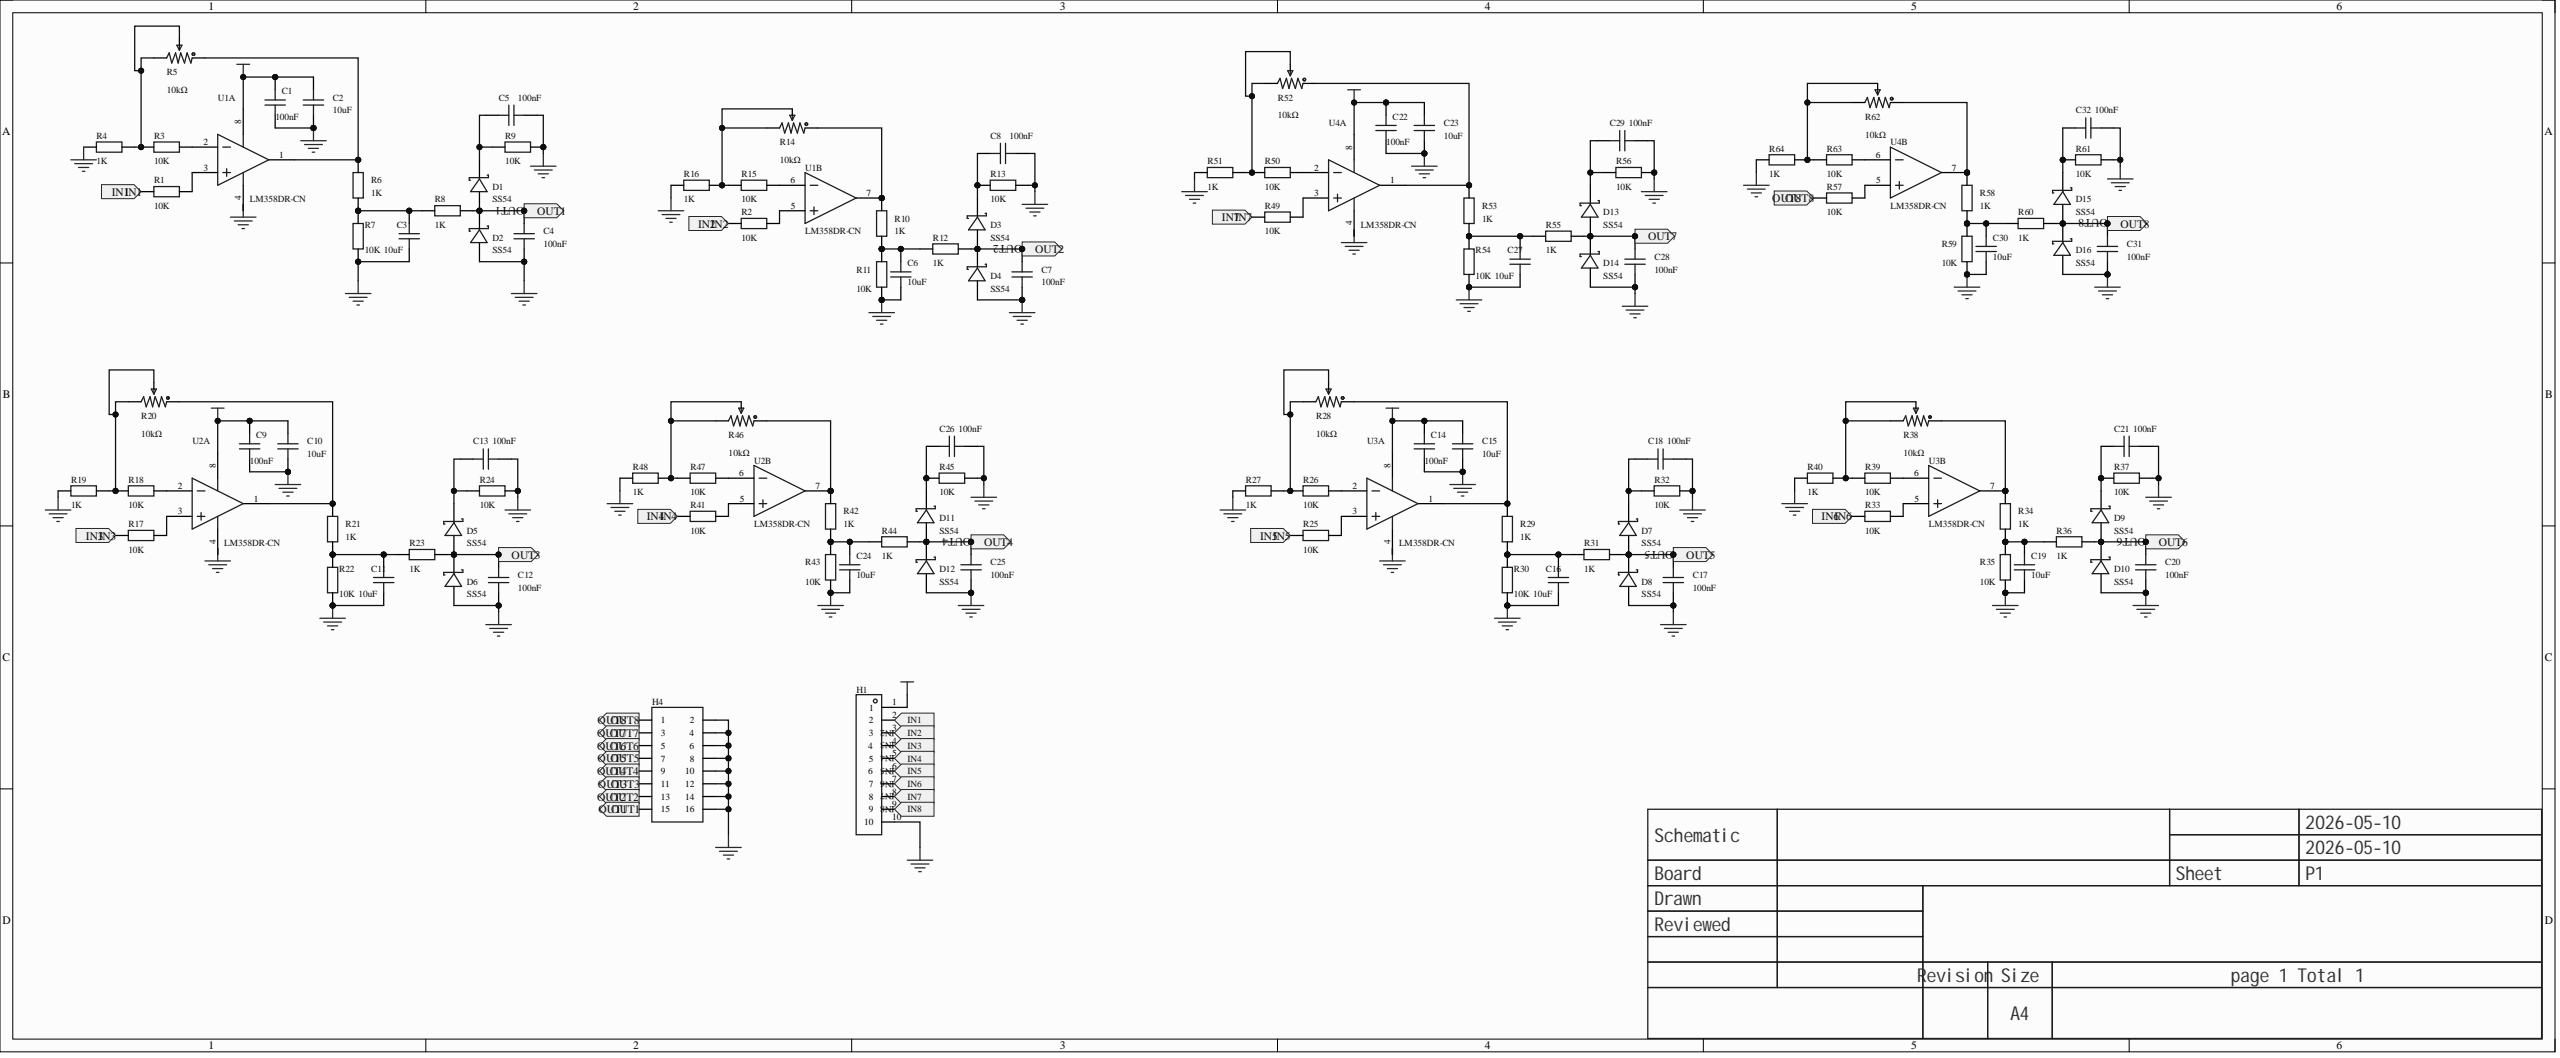Circuit board | Altium Designer | 118 parts | 65 nets
Bill of materials:
Comment,Description,Designator,Footprint,LibRef,Quantity
"100nF","","C1, C4, C5, C7, C8, C9, C12, C13, C14, C17, C18, C20, C21, C22, C25, C26, C28, C29, C31, C32","C0603","CAP_0603","20"
"10uF","","C2, C3, C6, C10, C11, C15, C16, C19, C23, C24, C27, C30","C0603","CAP_0603","12"
"SS54","Diode configuration: Single; Forward voltage (Vf): 550mV@5A; DC reverse voltage (Vr): 40V; Rectifier current: 5A;","D1, D2, D3, D4, D5, D6, D7, D8, D9, D10, D11, D12, D13, D14, D15, D16","SMA_L4.4-W2.8-LS5.4-R-RD","SS54_C22452","16"
"","","H1","HDR-TH_10P-P2.54-V-F","HDR-F_2.54_1x10P","1"
"","","H4","HDR-TH_16P-P2.54-V-F-R2-C8-S2.54-1","HDR-F_2.54_2x8","1"
"10K","","R1, R2, R3, R7, R9, R11, R13, R15, R17, R18, R22, R24, R25, R26, R30, R32, R33, R35, R37, R39, R41, R43, R45, R47, R49, R50, R54, R56, R57, R59, R61, R63","R0603","Res_0603","32"
"1K","","R4, R6, R8, R10, R12, R16, R19, R21, R23, R27, R29, R31, R34, R36, R40, R42, R44, R48, R51, R53, R55, R58, R60, R64","R0603","Res_0603","24"
"10kΩ","Resistance: 10kΩ; Tolerance: ±10%;","R5, R14, R20, R28, R38, R46, R52, R62","RES-ADJ-TH_3P-L10.0-W10.0-P2.50-L","3296W-1-103","8"
"LM358DR-CN","","U1, U2, U3, U4","SOIC-8_L4.9-W4.0-P1.27-LS6.0-BL","LM358DR-CN","4"
Netlist (Protel format):
[
C1
C0603
100nF



]
[
C2
C0603
10uF



]
[
C3
C0603
10uF



]
[
C4
C0603
100nF



]
[
C5
C0603
100nF



]
[
C6
C0603
10uF



]
[
C7
C0603
100nF



]
[
C8
C0603
100nF



]
[
C9
C0603
100nF



]
[
C10
C0603
10uF



]
[
C11
C0603
10uF



]
[
C12
C0603
100nF



]
[
C13
C0603
100nF



]
[
C14
C0603
100nF



]
[
C15
C0603
10uF



]
[
C16
C0603
10uF



]
[
C17
C0603
100nF



]
[
C18
C0603
100nF



]
[
C19
C0603
10uF



]
[
C20
C0603
100nF



]
[
C21
C0603
100nF



]
[
C22
C0603
100nF



]
[
C23
C0603
10uF



]
[
C24
C0603
10uF



]
[
C25
C0603
100nF



]
[
C26
C0603
100nF



]
[
C27
C0603
10uF



]
[
C28
C0603
100nF



]
[
C29
C0603
100nF



]
[
C30
C0603
10uF



]
[
C31
C0603
100nF



]
[
C32
C0603
100nF



]
[
D1
SMA_L4.4-W2.8-LS5.4-R-RD
SS54



]
[
D2
SMA_L4.4-W2.8-LS5.4-R-RD
SS54



]
[
D3
SMA_L4.4-W2.8-LS5.4-R-RD
SS54



]
[
D4
SMA_L4.4-W2.8-LS5.4-R-RD
SS54



]
[
D5
SMA_L4.4-W2.8-LS5.4-R-RD
SS54



]
[
D6
SMA_L4.4-W2.8-LS5.4-R-RD
SS54



]
[
D7
SMA_L4.4-W2.8-LS5.4-R-RD
SS54



]
[
D8
SMA_L4.4-W2.8-LS5.4-R-RD
SS54



]
[
D9
SMA_L4.4-W2.8-LS5.4-R-RD
SS54



]
[
D10
SMA_L4.4-W2.8-LS5.4-R-RD
SS54



]
[
D11
SMA_L4.4-W2.8-LS5.4-R-RD
SS54



]
[
D12
SMA_L4.4-W2.8-LS5.4-R-RD
SS54



]
[
D13
SMA_L4.4-W2.8-LS5.4-R-RD
SS54



]
[
D14
SMA_L4.4-W2.8-LS5.4-R-RD
SS54



]
[
D15
SMA_L4.4-W2.8-LS5.4-R-RD
SS54



]
[
D16
SMA_L4.4-W2.8-LS5.4-R-RD
SS54



]
[
H1
HDR-TH_10P-P2.54-V-F




]
[
H4
HDR-TH_16P-P2.54-V-F-R2-C8-S2.54-1




]
[
R1
R0603
10K



]
[
R2
R0603
10K



]
[
R3
R0603
10K



]
[
R4
R0603
1K



]
[
R5
RES-ADJ-TH_3P-L10.0-W10.0-P2.50-L
10kΩ



]
[
R6
R0603
1K



]
[
R7
R0603
10K



]
[
R8
R0603
1K



]
[
R9
R0603
10K



]
[
R10
R0603
1K



]
[
R11
R0603
10K



]
[
R12
R0603
1K



]
[
R13
R0603
10K



]
[
R14
RES-ADJ-TH_3P-L10.0-W10.0-P2.50-L
10kΩ



]
[
R15
R0603
10K



]
[
R16
R0603
1K



]
[
R17
R0603
10K



]
[
R18
R0603
10K



]
[
R19
R0603
1K



]
[
R20
RES-ADJ-TH_3P-L10.0-W10.0-P2.50-L
10kΩ



]
[
R21
R0603
1K



]
[
R22
R0603
10K



]
[
R23
R0603
1K



]
[
R24
R0603
10K



]
[
R25
R0603
10K



]
[
R26
R0603
10K



]
[
R27
R0603
1K



]
[
R28
RES-ADJ-TH_3P-L10.0-W10.0-P2.50-L
10kΩ



]
[
R29
R0603
1K



]
[
R30
R0603
10K



]
[
R31
R0603
1K



]
[
R32
R0603
10K



]
[
R33
R0603
10K



]
[
R34
R0603
1K



]
[
R35
R0603
10K



]
[
R36
R0603
1K



]
[
R37
R0603
10K



]
[
R38
RES-ADJ-TH_3P-L10.0-W10.0-P2.50-L
10kΩ



]
[
R39
R0603
10K



]
[
R40
R0603
1K



]
[
R41
R0603
10K



]
[
R42
R0603
1K



]
[
R43
R0603
10K



]
[
R44
R0603
1K



]
[
R45
R0603
10K



]
[
R46
RES-ADJ-TH_3P-L10.0-W10.0-P2.50-L
10kΩ



]
[
R47
R0603
10K



]
[
R48
R0603
1K



]
[
R49
R0603
10K



]
[
R50
R0603
10K



]
[
R51
R0603
1K



]
[
R52
RES-ADJ-TH_3P-L10.0-W10.0-P2.50-L
10kΩ



]
[
R53
R0603
1K



]
[
R54
R0603
10K



]
[
R55
R0603
1K



]
[
R56
R0603
10K



]
[
R57
R0603
10K



]
[
R58
R0603
1K



]
[
R59
R0603
10K



]
[
R60
R0603
1K



]
[
R61
R0603
10K



]
[
R62
RES-ADJ-TH_3P-L10.0-W10.0-P2.50-L
10kΩ



]
[
R63
R0603
10K



]
[
R64
R0603
1K



]
[
U1
SOIC-8_L4.9-W4.0-P1.27-LS6.0-BL
LM358DR-CN



]
[
U2
SOIC-8_L4.9-W4.0-P1.27-LS6.0-BL
LM358DR-CN



]
[
U3
SOIC-8_L4.9-W4.0-P1.27-LS6.0-BL
LM358DR-CN



]
[
U4
SOIC-8_L4.9-W4.0-P1.27-LS6.0-BL
LM358DR-CN



]
(
OUT8
C31-2
D15-1
D16-2
H4-1
R57-1
R60-2
)
(
OUT7
C28-2
D13-1
D14-2
H4-3
R55-2
)
(
OUT6
C20-2
D9-1
D10-2
H4-5
R36-2
)
(
OUT5
C17-2
D7-1
D8-2
H4-7
R31-2
)
(
OUT4
C25-2
D11-1
D12-2
H4-9
R44-2
)
(
OUT3
C12-2
D5-1
D6-2
H4-11
R23-2
)
(
OUT2
C7-2
D3-1
D4-2
H4-13
R12-2
)
(
OUT1
C4-2
D1-1
D2-2
H4-15
R8-2
)
(
NetR63_2
R63-2
U4-6
)
(
NetR62_2
R62-2
R62-3
R63-1
R64-2
)
(
NetR58_2
R58-2
R62-1
U4-7
)
(
NetR57_2
R57-2
U4-5
)
(
NetR52_1
R52-1
R53-2
U4-1
)
(
NetR50_2
R50-2
U4-2
)
(
NetR50_1
R50-1
R51-2
R52-2
R52-3
)
(
NetR49_2
R49-2
U4-3
)
(
NetR47_2
R47-2
U2-6
)
(
NetR46_2
R46-2
R46-3
R47-1
R48-2
)
(
NetR42_2
R42-2
R46-1
U2-7
)
(
NetR41_2
R41-2
U2-5
)
(
NetR39_2
R39-2
U3-6
)
(
NetR38_2
R38-2
R38-3
R39-1
R40-2
)
(
NetR34_2
R34-2
R38-1
U3-7
)
(
NetR33_2
R33-2
U3-5
)
(
NetR28_1
R28-1
R29-2
U3-1
)
(
NetR26_2
R26-2
U3-2
)
(
NetR26_1
R26-1
R27-2
R28-2
R28-3
)
(
NetR25_2
R25-2
U3-3
)
(
NetR20_1
R20-1
R21-2
U2-1
)
(
NetR18_2
R18-2
U2-2
)
(
NetR18_1
R18-1
R19-2
R20-2
R20-3
)
(
NetR17_2
R17-2
U2-3
)
(
NetR15_2
R15-2
U1-6
)
(
NetR14_2
R14-2
R14-3
R15-1
R16-2
)
(
NetR10_2
R10-2
R14-1
U1-7
)
(
NetR5_1
R5-1
R6-2
U1-1
)
(
NetR3_2
R3-2
U1-2
)
(
NetR3_1
R3-1
R4-2
R5-2
R5-3
)
(
NetR2_2
R2-2
U1-5
)
(
NetR1_2
R1-2
U1-3
)
(
NetC32_2
C32-2
D15-2
R61-1
)
(
NetC30_2
C30-2
R58-1
R59-2
R60-1
)
(
NetC29_2
C29-2
D13-2
R56-1
)
(
NetC27_2
C27-2
R53-1
R54-2
R55-1
)
(
NetC26_2
C26-2
D11-2
R45-1
)
(
NetC24_2
C24-2
R42-1
R43-2
R44-1
)
(
NetC21_2
C21-2
D9-2
R37-1
)
(
NetC19_2
C19-2
R34-1
R35-2
R36-1
)
(
NetC18_2
C18-2
D7-2
R32-1
)
(
NetC16_2
C16-2
R29-1
R30-2
R31-1
)
(
NetC13_2
C13-2
D5-2
R24-1
)
(
NetC11_2
C11-2
R21-1
R22-2
R23-1
)
(
NetC8_2
C8-2
D3-2
R13-1
)
(
NetC6_2
C6-2
R10-1
R11-2
R12-1
)
(
NetC5_2
C5-2
D1-2
R9-1
)
(
NetC3_2
C3-2
R6-1
R7-2
R8-1
)
(
IN7
H1-8
R49-1
)
(
IN6
H1-7
R33-1
)
(
IN5
H1-6
R25-1
)
(
IN4
H1-5
R41-1
)
(
IN3
H1-4
R17-1
)
(
IN2
H1-3
R2-1
)
(
IN1
H1-2
R1-1
)
(
GND
C1-1
C2-1
C3-1
C4-1
C5-1
C6-1
C7-1
C8-1
C9-1
C10-1
C11-1
C12-1
C13-1
C14-1
C15-1
C16-1
C17-1
C18-1
C19-1
C20-1
C21-1
C22-1
C23-1
C24-1
C25-1
C26-1
C27-1
C28-1
C29-1
C30-1
C31-1
C32-1
D2-1
D4-1
D6-1
D8-1
D10-1
D12-1
D14-1
D16-1
H1-10
H4-2
H4-4
H4-6
H4-8
H4-10
H4-12
H4-14
H4-16
R4-1
R7-1
R9-2
R11-1
R13-2
R16-1
R19-1
R22-1
R24-2
R27-1
R30-1
R32-2
R35-1
R37-2
R40-1
R43-1
R45-2
R48-1
R51-1
R54-1
R56-2
R59-1
R61-2
R64-1
U1-4
U2-4
U3-4
U4-4
)
(
+5V
C1-2
C2-2
C9-2
C10-2
C14-2
C15-2
C22-2
C23-2
H1-1
U1-8
U2-8
U3-8
U4-8
)